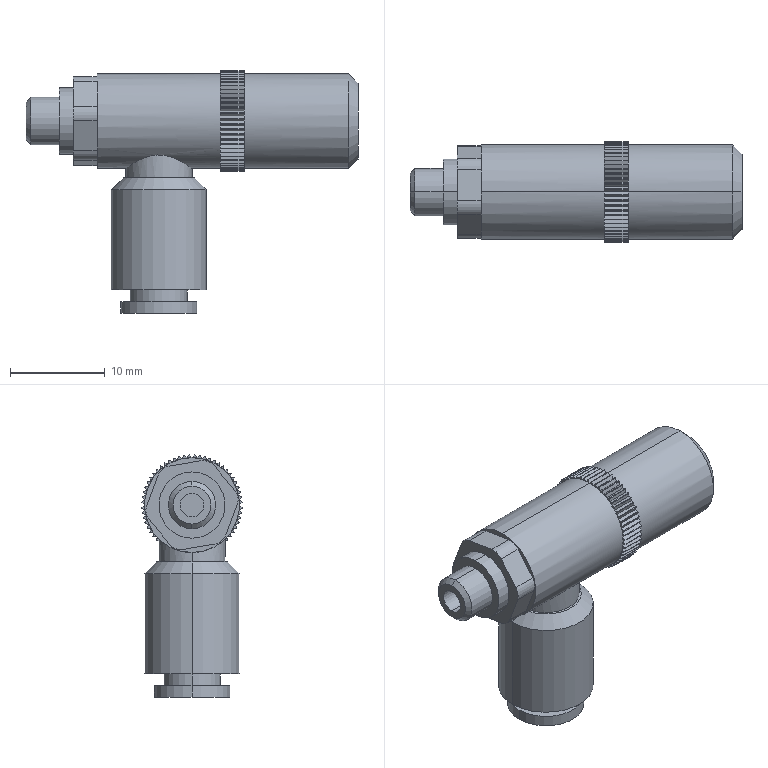Part | SolidWorks | features ICE 13, Chamfer 4, CirPattern 1, Extrusion 1, Fillet 1, RevCut 1, Revolution 1, Sweep 1 | 2 solids | 358 faces | box 35 x 10.589 x 25.544 mm | volume 3217 mm3 | plane 257 | cylinder 94 | cone 6 | sphere 1 | commonest cylinder face diameters 10.6 x60 10 x8 3 x7 7 x7 6 x4 2.5 x2